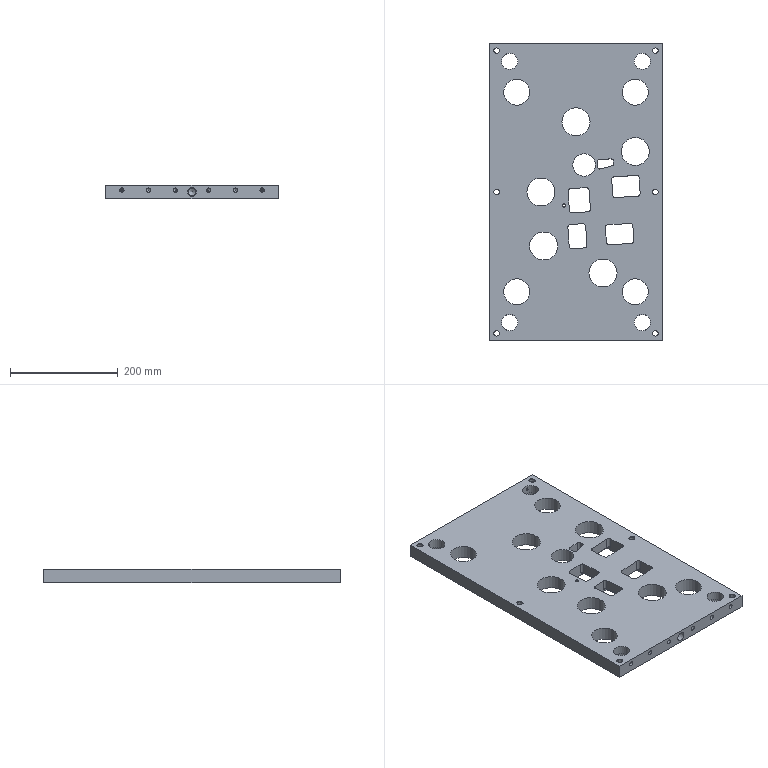Part | STEP file | 车灯-后视镜_id106_x_t | 1 solid | 173 faces | box 320 x 550 x 25 mm | volume 3596280 mm3 | cylinder 93 | plane 63 | cone 14 | spline 3 | commonest cylinder face diameters 10 x34 8 x16 6.9 x8 10.2 x6 12 x6 52 x5